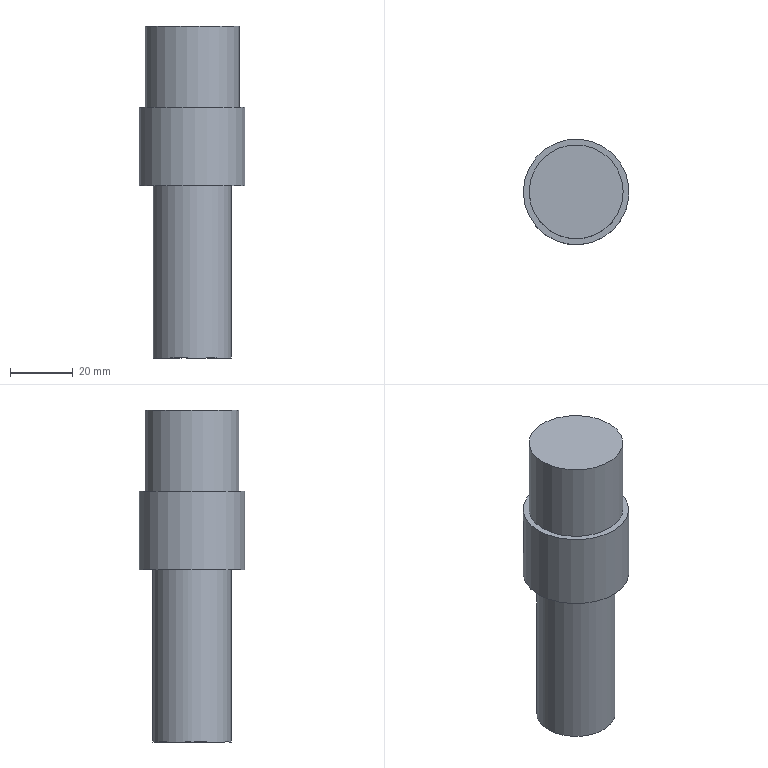Part | NX | features solid 2 | 1 solid | 7 faces | box 33.71 x 33.71 x 106 mm | volume 67688 mm3 | plane 4 | cylinder 3 | commonest cylinder face diameters 25 x1 30 x1 33.71 x1
STEP:
#1=CARTESIAN_POINT('',(-12.5,-440.,-145.));
#2=VERTEX_POINT('',#1);
#3=CARTESIAN_POINT('',(12.5,-440.,-145.));
#4=VERTEX_POINT('',#3);
#5=CARTESIAN_POINT('',(-12.5,-440.,-145.));
#6=CARTESIAN_POINT('',(-12.5,-444.419,-145.));
#7=CARTESIAN_POINT('',(-10.29,-450.29,-145.));
#8=CARTESIAN_POINT('',(-4.419,-452.5,-145.));
#9=CARTESIAN_POINT('',(4.419,-452.5,-145.));
#10=CARTESIAN_POINT('',(10.29,-450.29,-145.));
#11=CARTESIAN_POINT('',(12.5,-444.419,-145.));
#12=CARTESIAN_POINT('',(12.5,-440.,-145.));
#13=(BOUNDED_CURVE()B_SPLINE_CURVE(4,(#5,#6,#7,#8,#9,#10,#11,#12),.UNSPECIFIED.,.F.,.F.)B_SPLINE_CURVE_WITH_KNOTS((5,3,5),(0.5,0.75,1.),.UNSPECIFIED.)CURVE()GEOMETRIC_REPRESENTATION_ITEM()RATIONAL_B_SPLINE_CURVE((1.,1.,0.9428,1.,1.,0.9428,1.,1.))REPRESENTATION_ITEM(''));
#14=EDGE_CURVE('',#2,#4,#13,.T.);
#15=ORIENTED_EDGE('',*,*,#14,.F.);
#16=CARTESIAN_POINT('',(12.5,-440.,-145.));
#17=CARTESIAN_POINT('',(12.5,-435.581,-145.));
#18=CARTESIAN_POINT('',(10.29,-429.71,-145.));
#19=CARTESIAN_POINT('',(4.419,-427.5,-145.));
#20=CARTESIAN_POINT('',(-4.419,-427.5,-145.));
#21=CARTESIAN_POINT('',(-10.29,-429.71,-145.));
#22=CARTESIAN_POINT('',(-12.5,-435.581,-145.));
#23=CARTESIAN_POINT('',(-12.5,-440.,-145.));
#24=(BOUNDED_CURVE()B_SPLINE_CURVE(4,(#16,#17,#18,#19,#20,#21,#22,#23),.UNSPECIFIED.,.F.,.F.)B_SPLINE_CURVE_WITH_KNOTS((5,3,5),(0.,0.25,0.5),.UNSPECIFIED.)CURVE()GEOMETRIC_REPRESENTATION_ITEM()RATIONAL_B_SPLINE_CURVE((1.,1.,0.9428,1.,1.,0.9428,1.,1.))REPRESENTATION_ITEM(''));
#25=EDGE_CURVE('',#4,#2,#24,.T.);
#26=ORIENTED_EDGE('',*,*,#25,.F.);
#27=EDGE_LOOP('',(#15,#26));
#28=FACE_BOUND('',#27,.T.);
#29=CARTESIAN_POINT('',(12.5,-440.,-200.));
#30=VERTEX_POINT('',#29);
#31=CARTESIAN_POINT('',(-12.5,-440.,-200.));
#32=VERTEX_POINT('',#31);
#33=CARTESIAN_POINT('',(12.5,-440.,-200.));
#34=CARTESIAN_POINT('',(12.5,-435.581,-200.));
#35=CARTESIAN_POINT('',(10.29,-429.71,-200.));
#36=CARTESIAN_POINT('',(4.419,-427.5,-200.));
#37=CARTESIAN_POINT('',(-4.419,-427.5,-200.));
#38=CARTESIAN_POINT('',(-10.29,-429.71,-200.));
#39=CARTESIAN_POINT('',(-12.5,-435.581,-200.));
#40=CARTESIAN_POINT('',(-12.5,-440.,-200.));
#41=(BOUNDED_CURVE()B_SPLINE_CURVE(4,(#33,#34,#35,#36,#37,#38,#39,#40),.UNSPECIFIED.,.F.,.F.)B_SPLINE_CURVE_WITH_KNOTS((5,3,5),(0.,0.25,0.5),.UNSPECIFIED.)CURVE()GEOMETRIC_REPRESENTATION_ITEM()RATIONAL_B_SPLINE_CURVE((1.,1.,0.9428,1.,1.,0.9428,1.,1.))REPRESENTATION_ITEM(''));
#42=EDGE_CURVE('',#30,#32,#41,.T.);
#43=ORIENTED_EDGE('',*,*,#42,.T.);
#44=CARTESIAN_POINT('',(-12.5,-440.,-200.));
#45=CARTESIAN_POINT('',(-12.5,-444.419,-200.));
#46=CARTESIAN_POINT('',(-10.29,-450.29,-200.));
#47=CARTESIAN_POINT('',(-4.419,-452.5,-200.));
#48=CARTESIAN_POINT('',(4.419,-452.5,-200.));
#49=CARTESIAN_POINT('',(10.29,-450.29,-200.));
#50=CARTESIAN_POINT('',(12.5,-444.419,-200.));
#51=CARTESIAN_POINT('',(12.5,-440.,-200.));
#52=(BOUNDED_CURVE()B_SPLINE_CURVE(4,(#44,#45,#46,#47,#48,#49,#50,#51),.UNSPECIFIED.,.F.,.F.)B_SPLINE_CURVE_WITH_KNOTS((5,3,5),(0.5,0.75,1.),.UNSPECIFIED.)CURVE()GEOMETRIC_REPRESENTATION_ITEM()RATIONAL_B_SPLINE_CURVE((1.,1.,0.9428,1.,1.,0.9428,1.,1.))REPRESENTATION_ITEM(''));
#53=EDGE_CURVE('',#32,#30,#52,.T.);
#54=ORIENTED_EDGE('',*,*,#53,.T.);
#55=EDGE_LOOP('',(#43,#54));
#56=FACE_BOUND('',#55,.T.);
#57=CARTESIAN_POINT('',(0.,-440.,-200.));
#58=DIRECTION('',(0.,0.,1.));
#59=DIRECTION('',(-1.,0.,0.));
#60=AXIS2_PLACEMENT_3D('',#57,#58,#59);
#61=CYLINDRICAL_SURFACE('',#60,12.5);
#62=ADVANCED_FACE('',(#28,#56),#61,.T.);
#63=ORIENTED_EDGE('',*,*,#42,.F.);
#64=ORIENTED_EDGE('',*,*,#53,.F.);
#65=EDGE_LOOP('',(#63,#64));
#66=FACE_BOUND('',#65,.T.);
#67=CARTESIAN_POINT('',(0.,-427.5,-200.));
#68=DIRECTION('',(0.,0.,1.));
#69=DIRECTION('',(-1.,0.,0.));
#70=AXIS2_PLACEMENT_3D('',#67,#68,#69);
#71=PLANE('',#70);
#72=ADVANCED_FACE('',(#66),#71,.F.);
#73=CARTESIAN_POINT('',(-16.855,-440.,-145.));
#74=VERTEX_POINT('',#73);
#75=CARTESIAN_POINT('',(0.,-440.,-145.));
#76=DIRECTION('',(0.,0.,1.));
#77=DIRECTION('',(-1.,0.,0.));
#78=AXIS2_PLACEMENT_3D('',#75,#76,#77);
#79=CIRCLE('',#78,16.855);
#80=EDGE_CURVE('',#74,#74,#79,.T.);
#81=ORIENTED_EDGE('',*,*,#80,.T.);
#82=EDGE_LOOP('',(#81));
#83=FACE_BOUND('',#82,.T.);
#84=CARTESIAN_POINT('',(-16.855,-440.,-120.));
#85=VERTEX_POINT('',#84);
#86=CARTESIAN_POINT('',(0.,-440.,-120.));
#87=DIRECTION('',(0.,0.,1.));
#88=DIRECTION('',(-1.,0.,0.));
#89=AXIS2_PLACEMENT_3D('',#86,#87,#88);
#90=CIRCLE('',#89,16.855);
#91=EDGE_CURVE('',#85,#85,#90,.T.);
#92=ORIENTED_EDGE('',*,*,#91,.F.);
#93=EDGE_LOOP('',(#92));
#94=FACE_BOUND('',#93,.T.);
#95=CARTESIAN_POINT('',(0.,-440.,-145.));
#96=DIRECTION('',(0.,0.,1.));
#97=DIRECTION('',(-1.,0.,0.));
#98=AXIS2_PLACEMENT_3D('',#95,#96,#97);
#99=CYLINDRICAL_SURFACE('',#98,16.855);
#100=ADVANCED_FACE('',(#83,#94),#99,.T.);
#101=ORIENTED_EDGE('',*,*,#14,.T.);
#102=ORIENTED_EDGE('',*,*,#25,.T.);
#103=EDGE_LOOP('',(#101,#102));
#104=FACE_BOUND('',#103,.T.);
#105=ORIENTED_EDGE('',*,*,#80,.F.);
#106=EDGE_LOOP('',(#105));
#107=FACE_BOUND('',#106,.T.);
#108=CARTESIAN_POINT('',(0.,-440.,-145.));
#109=DIRECTION('',(0.,0.,-1.));
#110=DIRECTION('',(1.,0.,0.));
#111=AXIS2_PLACEMENT_3D('',#108,#109,#110);
#112=PLANE('',#111);
#113=ADVANCED_FACE('',(#104,#107),#112,.T.);
#114=CARTESIAN_POINT('',(-15.,-440.,-120.));
#115=VERTEX_POINT('',#114);
#116=CARTESIAN_POINT('',(0.,-440.,-120.));
#117=DIRECTION('',(0.,0.,1.));
#118=DIRECTION('',(-1.,0.,0.));
#119=AXIS2_PLACEMENT_3D('',#116,#117,#118);
#120=CIRCLE('',#119,15.);
#121=EDGE_CURVE('',#115,#115,#120,.T.);
#122=ORIENTED_EDGE('',*,*,#121,.F.);
#123=EDGE_LOOP('',(#122));
#124=FACE_BOUND('',#123,.T.);
#125=ORIENTED_EDGE('',*,*,#91,.T.);
#126=EDGE_LOOP('',(#125));
#127=FACE_BOUND('',#126,.T.);
#128=CARTESIAN_POINT('',(0.,-440.,-120.));
#129=DIRECTION('',(0.,0.,-1.));
#130=DIRECTION('',(1.,0.,0.));
#131=AXIS2_PLACEMENT_3D('',#128,#129,#130);
#132=PLANE('',#131);
#133=ADVANCED_FACE('',(#124,#127),#132,.F.);
#134=CARTESIAN_POINT('',(15.,-440.,-94.));
#135=VERTEX_POINT('',#134);
#136=CARTESIAN_POINT('',(0.,-440.,-94.));
#137=DIRECTION('',(0.,0.,1.));
#138=DIRECTION('',(1.,0.,0.));
#139=AXIS2_PLACEMENT_3D('',#136,#137,#138);
#140=CIRCLE('',#139,15.);
#141=EDGE_CURVE('',#135,#135,#140,.T.);
#142=ORIENTED_EDGE('',*,*,#141,.F.);
#143=EDGE_LOOP('',(#142));
#144=FACE_BOUND('',#143,.T.);
#145=ORIENTED_EDGE('',*,*,#121,.T.);
#146=EDGE_LOOP('',(#145));
#147=FACE_BOUND('',#146,.T.);
#148=CARTESIAN_POINT('',(0.,-440.,-85.));
#149=DIRECTION('',(0.,0.,-1.));
#150=DIRECTION('',(1.,0.,0.));
#151=AXIS2_PLACEMENT_3D('',#148,#149,#150);
#152=CYLINDRICAL_SURFACE('',#151,15.);
#153=ADVANCED_FACE('',(#144,#147),#152,.T.);
#154=ORIENTED_EDGE('',*,*,#141,.T.);
#155=EDGE_LOOP('',(#154));
#156=FACE_BOUND('',#155,.T.);
#157=CARTESIAN_POINT('',(-80.,-440.,-94.));
#158=DIRECTION('',(0.,0.,-1.));
#159=DIRECTION('',(1.,0.,0.));
#160=AXIS2_PLACEMENT_3D('',#157,#158,#159);
#161=PLANE('',#160);
#162=ADVANCED_FACE('',(#156),#161,.F.);
#163=CLOSED_SHELL('',(#62,#72,#100,#113,#133,#153,#162));
#164=MANIFOLD_SOLID_BREP('',#163);
#165=(LENGTH_UNIT()NAMED_UNIT(*)SI_UNIT(.MILLI.,.METRE.));
#166=UNCERTAINTY_MEASURE_WITH_UNIT(LENGTH_MEASURE(0.00001),#165,'','');
#167=(NAMED_UNIT(*)PLANE_ANGLE_UNIT()SI_UNIT($,.RADIAN.));
#168=(NAMED_UNIT(*)SI_UNIT($,.STERADIAN.)SOLID_ANGLE_UNIT());
#169=(GEOMETRIC_REPRESENTATION_CONTEXT(3)GLOBAL_UNCERTAINTY_ASSIGNED_CONTEXT((#166))GLOBAL_UNIT_ASSIGNED_CONTEXT((#165,#167,#168))REPRESENTATION_CONTEXT('',''));
#170=ADVANCED_BREP_SHAPE_REPRESENTATION('',(#164),#169);